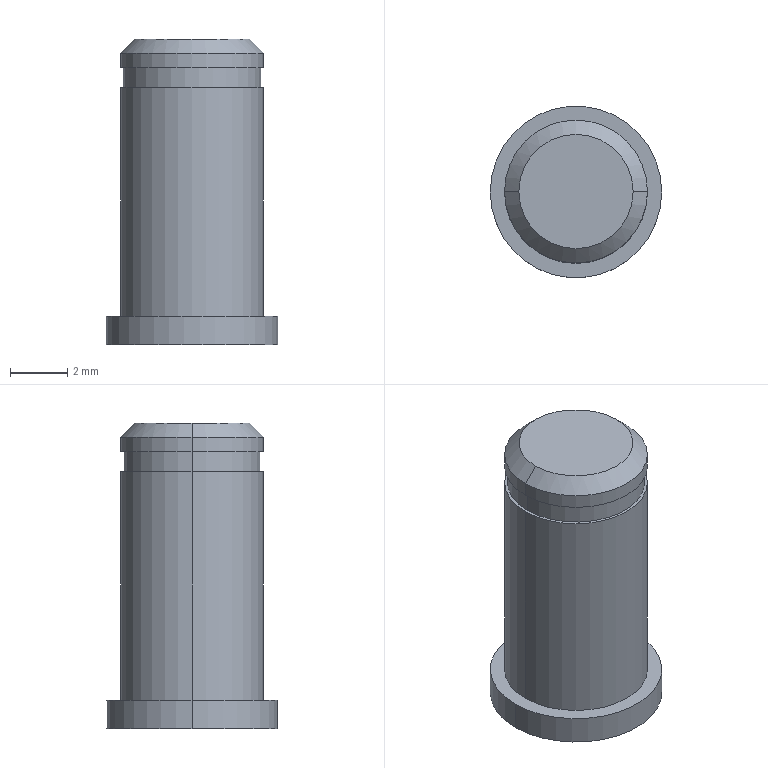Part | STEP file | PN_0105 Mount electronic clip sensor 3 | 1 solid | 15 faces | box 6 x 6 x 10.7 mm | volume 215.823 mm3 | cylinder 8 | plane 5 | cone 2 | commonest cylinder face diameters 5 x4 4.8 x2 6 x2
STEP:
#1=CARTESIAN_POINT('',(0.,0.,0.));
#2=DIRECTION('',(0.,0.,1.));
#3=DIRECTION('',(1.,0.,0.));
#4=AXIS2_PLACEMENT_3D('',#1,#2,#3);
#5=CARTESIAN_POINT('',(2.,0.,10.7));
#6=VERTEX_POINT('',#5);
#7=CARTESIAN_POINT('',(-2.,0.,10.7));
#8=VERTEX_POINT('',#7);
#9=CARTESIAN_POINT('',(0.,0.,10.7));
#10=DIRECTION('',(0.,0.,1.));
#11=DIRECTION('',(1.,0.,0.));
#12=AXIS2_PLACEMENT_3D('',#9,#10,#11);
#13=CIRCLE('',#12,2.);
#14=CARTESIAN_POINT('',(0.,0.,10.7));
#15=DIRECTION('',(0.,0.,-1.));
#16=DIRECTION('',(-1.,0.,0.));
#17=AXIS2_PLACEMENT_3D('',#14,#15,#16);
#18=CONICAL_SURFACE('',#17,2.,0.7854);
#19=CARTESIAN_POINT('',(3.142,0.));
#20=DIRECTION('',(-1.,0.));
#21=VECTOR('',#20,1.);
#22=LINE('',#19,#21);
#23=(GEOMETRIC_REPRESENTATION_CONTEXT(2)PARAMETRIC_REPRESENTATION_CONTEXT()REPRESENTATION_CONTEXT('',''));
#24=DEFINITIONAL_REPRESENTATION('',(#22),#23);
#25=PCURVE('',#18,#24);
#26=CARTESIAN_POINT('',(0.,0.,10.7));
#27=DIRECTION('',(0.,0.,1.));
#28=DIRECTION('',(1.,0.,0.));
#29=AXIS2_PLACEMENT_3D('',#26,#27,#28);
#30=PLANE('',#29);
#31=CARTESIAN_POINT('',(0.,0.));
#32=DIRECTION('',(1.,0.));
#33=AXIS2_PLACEMENT_2D('',#31,#32);
#34=CIRCLE('',#33,2.);
#35=(GEOMETRIC_REPRESENTATION_CONTEXT(2)PARAMETRIC_REPRESENTATION_CONTEXT()REPRESENTATION_CONTEXT('',''));
#36=DEFINITIONAL_REPRESENTATION('',(#34),#35);
#37=PCURVE('',#30,#36);
#38=SURFACE_CURVE('',#13,(#25,#37),.PCURVE_S1.);
#39=EDGE_CURVE('',#6,#8,#38,.T.);
#40=ORIENTED_EDGE('',*,*,#39,.F.);
#41=CARTESIAN_POINT('',(2.5,0.,10.2));
#42=VERTEX_POINT('',#41);
#43=CARTESIAN_POINT('',(2.,0.,10.7));
#44=DIRECTION('',(0.7071,0.,-0.7071));
#45=VECTOR('',#44,1.);
#46=LINE('',#43,#45);
#47=CARTESIAN_POINT('',(3.142,0.));
#48=DIRECTION('',(0.,1.));
#49=VECTOR('',#48,1.);
#50=LINE('',#47,#49);
#51=(GEOMETRIC_REPRESENTATION_CONTEXT(2)PARAMETRIC_REPRESENTATION_CONTEXT()REPRESENTATION_CONTEXT('',''));
#52=DEFINITIONAL_REPRESENTATION('',(#50),#51);
#53=PCURVE('',#18,#52);
#54=CARTESIAN_POINT('',(0.,0.,10.7));
#55=DIRECTION('',(0.,0.,-1.));
#56=DIRECTION('',(-1.,0.,0.));
#57=AXIS2_PLACEMENT_3D('',#54,#55,#56);
#58=CONICAL_SURFACE('',#57,2.,0.7854);
#59=CARTESIAN_POINT('',(3.142,0.));
#60=DIRECTION('',(0.,1.));
#61=VECTOR('',#60,1.);
#62=LINE('',#59,#61);
#63=(GEOMETRIC_REPRESENTATION_CONTEXT(2)PARAMETRIC_REPRESENTATION_CONTEXT()REPRESENTATION_CONTEXT('',''));
#64=DEFINITIONAL_REPRESENTATION('',(#62),#63);
#65=PCURVE('',#58,#64);
#66=SURFACE_CURVE('',#46,(#53,#65),.PCURVE_S1.);
#67=EDGE_CURVE('',#6,#42,#66,.T.);
#68=ORIENTED_EDGE('',*,*,#67,.T.);
#69=CARTESIAN_POINT('',(-2.5,0.,10.2));
#70=VERTEX_POINT('',#69);
#71=CARTESIAN_POINT('',(0.,0.,10.2));
#72=DIRECTION('',(0.,0.,-1.));
#73=DIRECTION('',(1.,0.,0.));
#74=AXIS2_PLACEMENT_3D('',#71,#72,#73);
#75=CIRCLE('',#74,2.5);
#76=CARTESIAN_POINT('',(-3.142,0.5));
#77=DIRECTION('',(1.,0.));
#78=VECTOR('',#77,1.);
#79=LINE('',#76,#78);
#80=(GEOMETRIC_REPRESENTATION_CONTEXT(2)PARAMETRIC_REPRESENTATION_CONTEXT()REPRESENTATION_CONTEXT('',''));
#81=DEFINITIONAL_REPRESENTATION('',(#79),#80);
#82=PCURVE('',#18,#81);
#83=CARTESIAN_POINT('',(0.,0.,10.7));
#84=DIRECTION('',(0.,0.,-1.));
#85=DIRECTION('',(-1.,0.,0.));
#86=AXIS2_PLACEMENT_3D('',#83,#84,#85);
#87=CYLINDRICAL_SURFACE('',#86,2.5);
#88=CARTESIAN_POINT('',(-3.142,0.5));
#89=DIRECTION('',(1.,0.));
#90=VECTOR('',#89,1.);
#91=LINE('',#88,#90);
#92=(GEOMETRIC_REPRESENTATION_CONTEXT(2)PARAMETRIC_REPRESENTATION_CONTEXT()REPRESENTATION_CONTEXT('',''));
#93=DEFINITIONAL_REPRESENTATION('',(#91),#92);
#94=PCURVE('',#87,#93);
#95=SURFACE_CURVE('',#75,(#82,#94),.PCURVE_S1.);
#96=EDGE_CURVE('',#70,#42,#95,.T.);
#97=ORIENTED_EDGE('',*,*,#96,.F.);
#98=CARTESIAN_POINT('',(-2.,0.,10.7));
#99=DIRECTION('',(-0.7071,0.,-0.7071));
#100=VECTOR('',#99,1.);
#101=LINE('',#98,#100);
#102=CARTESIAN_POINT('',(0.,0.));
#103=DIRECTION('',(0.,1.));
#104=VECTOR('',#103,1.);
#105=LINE('',#102,#104);
#106=(GEOMETRIC_REPRESENTATION_CONTEXT(2)PARAMETRIC_REPRESENTATION_CONTEXT()REPRESENTATION_CONTEXT('',''));
#107=DEFINITIONAL_REPRESENTATION('',(#105),#106);
#108=PCURVE('',#18,#107);
#109=CARTESIAN_POINT('',(6.283,0.));
#110=DIRECTION('',(0.,1.));
#111=VECTOR('',#110,1.);
#112=LINE('',#109,#111);
#113=(GEOMETRIC_REPRESENTATION_CONTEXT(2)PARAMETRIC_REPRESENTATION_CONTEXT()REPRESENTATION_CONTEXT('',''));
#114=DEFINITIONAL_REPRESENTATION('',(#112),#113);
#115=PCURVE('',#58,#114);
#116=SURFACE_CURVE('',#101,(#108,#115),.PCURVE_S1.);
#117=EDGE_CURVE('',#8,#70,#116,.T.);
#118=ORIENTED_EDGE('',*,*,#117,.F.);
#119=EDGE_LOOP('',(#40,#68,#97,#118));
#120=FACE_BOUND('',#119,.T.);
#121=ADVANCED_FACE('',(#120),#18,.T.);
#122=ORIENTED_EDGE('',*,*,#96,.T.);
#123=CARTESIAN_POINT('',(2.5,0.,9.7));
#124=VERTEX_POINT('',#123);
#125=CARTESIAN_POINT('',(2.5,0.,10.7));
#126=DIRECTION('',(0.,0.,-1.));
#127=VECTOR('',#126,1.);
#128=LINE('',#125,#127);
#129=CARTESIAN_POINT('',(3.142,0.));
#130=DIRECTION('',(0.,1.));
#131=VECTOR('',#130,1.);
#132=LINE('',#129,#131);
#133=(GEOMETRIC_REPRESENTATION_CONTEXT(2)PARAMETRIC_REPRESENTATION_CONTEXT()REPRESENTATION_CONTEXT('',''));
#134=DEFINITIONAL_REPRESENTATION('',(#132),#133);
#135=PCURVE('',#87,#134);
#136=CARTESIAN_POINT('',(0.,0.,10.7));
#137=DIRECTION('',(0.,0.,-1.));
#138=DIRECTION('',(-1.,0.,0.));
#139=AXIS2_PLACEMENT_3D('',#136,#137,#138);
#140=CYLINDRICAL_SURFACE('',#139,2.5);
#141=CARTESIAN_POINT('',(3.142,0.));
#142=DIRECTION('',(0.,1.));
#143=VECTOR('',#142,1.);
#144=LINE('',#141,#143);
#145=(GEOMETRIC_REPRESENTATION_CONTEXT(2)PARAMETRIC_REPRESENTATION_CONTEXT()REPRESENTATION_CONTEXT('',''));
#146=DEFINITIONAL_REPRESENTATION('',(#144),#145);
#147=PCURVE('',#140,#146);
#148=SURFACE_CURVE('',#128,(#135,#147),.PCURVE_S1.);
#149=EDGE_CURVE('',#42,#124,#148,.T.);
#150=ORIENTED_EDGE('',*,*,#149,.T.);
#151=CARTESIAN_POINT('',(-2.5,0.,9.7));
#152=VERTEX_POINT('',#151);
#153=CARTESIAN_POINT('',(0.,0.,9.7));
#154=DIRECTION('',(0.,0.,1.));
#155=DIRECTION('',(1.,0.,0.));
#156=AXIS2_PLACEMENT_3D('',#153,#154,#155);
#157=CIRCLE('',#156,2.5);
#158=CARTESIAN_POINT('',(3.142,1.));
#159=DIRECTION('',(-1.,0.));
#160=VECTOR('',#159,1.);
#161=LINE('',#158,#160);
#162=(GEOMETRIC_REPRESENTATION_CONTEXT(2)PARAMETRIC_REPRESENTATION_CONTEXT()REPRESENTATION_CONTEXT('',''));
#163=DEFINITIONAL_REPRESENTATION('',(#161),#162);
#164=PCURVE('',#87,#163);
#165=CARTESIAN_POINT('',(0.,0.,9.7));
#166=DIRECTION('',(0.,0.,1.));
#167=DIRECTION('',(1.,0.,0.));
#168=AXIS2_PLACEMENT_3D('',#165,#166,#167);
#169=PLANE('',#168);
#170=CARTESIAN_POINT('',(0.,0.));
#171=DIRECTION('',(1.,0.));
#172=AXIS2_PLACEMENT_2D('',#170,#171);
#173=CIRCLE('',#172,2.5);
#174=(GEOMETRIC_REPRESENTATION_CONTEXT(2)PARAMETRIC_REPRESENTATION_CONTEXT()REPRESENTATION_CONTEXT('',''));
#175=DEFINITIONAL_REPRESENTATION('',(#173),#174);
#176=PCURVE('',#169,#175);
#177=SURFACE_CURVE('',#157,(#164,#176),.PCURVE_S1.);
#178=EDGE_CURVE('',#124,#152,#177,.T.);
#179=ORIENTED_EDGE('',*,*,#178,.T.);
#180=CARTESIAN_POINT('',(-2.5,0.,10.7));
#181=DIRECTION('',(0.,0.,-1.));
#182=VECTOR('',#181,1.);
#183=LINE('',#180,#182);
#184=CARTESIAN_POINT('',(0.,0.));
#185=DIRECTION('',(0.,1.));
#186=VECTOR('',#185,1.);
#187=LINE('',#184,#186);
#188=(GEOMETRIC_REPRESENTATION_CONTEXT(2)PARAMETRIC_REPRESENTATION_CONTEXT()REPRESENTATION_CONTEXT('',''));
#189=DEFINITIONAL_REPRESENTATION('',(#187),#188);
#190=PCURVE('',#87,#189);
#191=CARTESIAN_POINT('',(6.283,0.));
#192=DIRECTION('',(0.,1.));
#193=VECTOR('',#192,1.);
#194=LINE('',#191,#193);
#195=(GEOMETRIC_REPRESENTATION_CONTEXT(2)PARAMETRIC_REPRESENTATION_CONTEXT()REPRESENTATION_CONTEXT('',''));
#196=DEFINITIONAL_REPRESENTATION('',(#194),#195);
#197=PCURVE('',#140,#196);
#198=SURFACE_CURVE('',#183,(#190,#197),.PCURVE_S1.);
#199=EDGE_CURVE('',#70,#152,#198,.T.);
#200=ORIENTED_EDGE('',*,*,#199,.F.);
#201=EDGE_LOOP('',(#122,#150,#179,#200));
#202=FACE_BOUND('',#201,.T.);
#203=ADVANCED_FACE('',(#202),#87,.T.);
#204=CARTESIAN_POINT('',(2.4,0.,9.7));
#205=VERTEX_POINT('',#204);
#206=CARTESIAN_POINT('',(-2.4,0.,9.7));
#207=VERTEX_POINT('',#206);
#208=CARTESIAN_POINT('',(0.,0.,9.7));
#209=DIRECTION('',(0.,0.,1.));
#210=DIRECTION('',(1.,0.,0.));
#211=AXIS2_PLACEMENT_3D('',#208,#209,#210);
#212=CIRCLE('',#211,2.4);
#213=CARTESIAN_POINT('',(0.,0.,9.7));
#214=DIRECTION('',(0.,0.,-1.));
#215=DIRECTION('',(-1.,0.,0.));
#216=AXIS2_PLACEMENT_3D('',#213,#214,#215);
#217=CYLINDRICAL_SURFACE('',#216,2.4);
#218=CARTESIAN_POINT('',(3.142,0.));
#219=DIRECTION('',(-1.,0.));
#220=VECTOR('',#219,1.);
#221=LINE('',#218,#220);
#222=(GEOMETRIC_REPRESENTATION_CONTEXT(2)PARAMETRIC_REPRESENTATION_CONTEXT()REPRESENTATION_CONTEXT('',''));
#223=DEFINITIONAL_REPRESENTATION('',(#221),#222);
#224=PCURVE('',#217,#223);
#225=CARTESIAN_POINT('',(0.,0.));
#226=DIRECTION('',(1.,0.));
#227=AXIS2_PLACEMENT_2D('',#225,#226);
#228=CIRCLE('',#227,2.4);
#229=(GEOMETRIC_REPRESENTATION_CONTEXT(2)PARAMETRIC_REPRESENTATION_CONTEXT()REPRESENTATION_CONTEXT('',''));
#230=DEFINITIONAL_REPRESENTATION('',(#228),#229);
#231=PCURVE('',#169,#230);
#232=SURFACE_CURVE('',#212,(#224,#231),.PCURVE_S1.);
#233=EDGE_CURVE('',#205,#207,#232,.T.);
#234=ORIENTED_EDGE('',*,*,#233,.F.);
#235=CARTESIAN_POINT('',(2.4,0.,9.));
#236=VERTEX_POINT('',#235);
#237=CARTESIAN_POINT('',(2.4,0.,9.7));
#238=DIRECTION('',(0.,0.,-1.));
#239=VECTOR('',#238,1.);
#240=LINE('',#237,#239);
#241=CARTESIAN_POINT('',(3.142,0.));
#242=DIRECTION('',(0.,1.));
#243=VECTOR('',#242,1.);
#244=LINE('',#241,#243);
#245=(GEOMETRIC_REPRESENTATION_CONTEXT(2)PARAMETRIC_REPRESENTATION_CONTEXT()REPRESENTATION_CONTEXT('',''));
#246=DEFINITIONAL_REPRESENTATION('',(#244),#245);
#247=PCURVE('',#217,#246);
#248=CARTESIAN_POINT('',(0.,0.,9.7));
#249=DIRECTION('',(0.,0.,-1.));
#250=DIRECTION('',(-1.,0.,0.));
#251=AXIS2_PLACEMENT_3D('',#248,#249,#250);
#252=CYLINDRICAL_SURFACE('',#251,2.4);
#253=CARTESIAN_POINT('',(3.142,0.));
#254=DIRECTION('',(0.,1.));
#255=VECTOR('',#254,1.);
#256=LINE('',#253,#255);
#257=(GEOMETRIC_REPRESENTATION_CONTEXT(2)PARAMETRIC_REPRESENTATION_CONTEXT()REPRESENTATION_CONTEXT('',''));
#258=DEFINITIONAL_REPRESENTATION('',(#256),#257);
#259=PCURVE('',#252,#258);
#260=SURFACE_CURVE('',#240,(#247,#259),.PCURVE_S1.);
#261=EDGE_CURVE('',#205,#236,#260,.T.);
#262=ORIENTED_EDGE('',*,*,#261,.T.);
#263=CARTESIAN_POINT('',(-2.4,0.,9.));
#264=VERTEX_POINT('',#263);
#265=CARTESIAN_POINT('',(0.,0.,9.));
#266=DIRECTION('',(0.,0.,1.));
#267=DIRECTION('',(1.,0.,0.));
#268=AXIS2_PLACEMENT_3D('',#265,#266,#267);
#269=CIRCLE('',#268,2.4);
#270=CARTESIAN_POINT('',(3.142,0.7));
#271=DIRECTION('',(-1.,0.));
#272=VECTOR('',#271,1.);
#273=LINE('',#270,#272);
#274=(GEOMETRIC_REPRESENTATION_CONTEXT(2)PARAMETRIC_REPRESENTATION_CONTEXT()REPRESENTATION_CONTEXT('',''));
#275=DEFINITIONAL_REPRESENTATION('',(#273),#274);
#276=PCURVE('',#217,#275);
#277=CARTESIAN_POINT('',(0.,0.,9.));
#278=DIRECTION('',(0.,0.,1.));
#279=DIRECTION('',(1.,0.,0.));
#280=AXIS2_PLACEMENT_3D('',#277,#278,#279);
#281=PLANE('',#280);
#282=CARTESIAN_POINT('',(0.,0.));
#283=DIRECTION('',(1.,0.));
#284=AXIS2_PLACEMENT_2D('',#282,#283);
#285=CIRCLE('',#284,2.4);
#286=(GEOMETRIC_REPRESENTATION_CONTEXT(2)PARAMETRIC_REPRESENTATION_CONTEXT()REPRESENTATION_CONTEXT('',''));
#287=DEFINITIONAL_REPRESENTATION('',(#285),#286);
#288=PCURVE('',#281,#287);
#289=SURFACE_CURVE('',#269,(#276,#288),.PCURVE_S1.);
#290=EDGE_CURVE('',#236,#264,#289,.T.);
#291=ORIENTED_EDGE('',*,*,#290,.T.);
#292=CARTESIAN_POINT('',(-2.4,0.,9.7));
#293=DIRECTION('',(0.,0.,-1.));
#294=VECTOR('',#293,1.);
#295=LINE('',#292,#294);
#296=CARTESIAN_POINT('',(0.,0.));
#297=DIRECTION('',(0.,1.));
#298=VECTOR('',#297,1.);
#299=LINE('',#296,#298);
#300=(GEOMETRIC_REPRESENTATION_CONTEXT(2)PARAMETRIC_REPRESENTATION_CONTEXT()REPRESENTATION_CONTEXT('',''));
#301=DEFINITIONAL_REPRESENTATION('',(#299),#300);
#302=PCURVE('',#217,#301);
#303=CARTESIAN_POINT('',(6.283,0.));
#304=DIRECTION('',(0.,1.));
#305=VECTOR('',#304,1.);
#306=LINE('',#303,#305);
#307=(GEOMETRIC_REPRESENTATION_CONTEXT(2)PARAMETRIC_REPRESENTATION_CONTEXT()REPRESENTATION_CONTEXT('',''));
#308=DEFINITIONAL_REPRESENTATION('',(#306),#307);
#309=PCURVE('',#252,#308);
#310=SURFACE_CURVE('',#295,(#302,#309),.PCURVE_S1.);
#311=EDGE_CURVE('',#207,#264,#310,.T.);
#312=ORIENTED_EDGE('',*,*,#311,.F.);
#313=EDGE_LOOP('',(#234,#262,#291,#312));
#314=FACE_BOUND('',#313,.T.);
#315=ADVANCED_FACE('',(#314),#217,.T.);
#316=CARTESIAN_POINT('',(2.5,0.,9.));
#317=VERTEX_POINT('',#316);
#318=CARTESIAN_POINT('',(-2.5,0.,9.));
#319=VERTEX_POINT('',#318);
#320=CARTESIAN_POINT('',(0.,0.,9.));
#321=DIRECTION('',(0.,0.,1.));
#322=DIRECTION('',(1.,0.,0.));
#323=AXIS2_PLACEMENT_3D('',#320,#321,#322);
#324=CIRCLE('',#323,2.5);
#325=CARTESIAN_POINT('',(0.,0.,9.));
#326=DIRECTION('',(0.,0.,-1.));
#327=DIRECTION('',(-1.,0.,0.));
#328=AXIS2_PLACEMENT_3D('',#325,#326,#327);
#329=CYLINDRICAL_SURFACE('',#328,2.5);
#330=CARTESIAN_POINT('',(3.142,0.));
#331=DIRECTION('',(-1.,0.));
#332=VECTOR('',#331,1.);
#333=LINE('',#330,#332);
#334=(GEOMETRIC_REPRESENTATION_CONTEXT(2)PARAMETRIC_REPRESENTATION_CONTEXT()REPRESENTATION_CONTEXT('',''));
#335=DEFINITIONAL_REPRESENTATION('',(#333),#334);
#336=PCURVE('',#329,#335);
#337=CARTESIAN_POINT('',(0.,0.));
#338=DIRECTION('',(1.,0.));
#339=AXIS2_PLACEMENT_2D('',#337,#338);
#340=CIRCLE('',#339,2.5);
#341=(GEOMETRIC_REPRESENTATION_CONTEXT(2)PARAMETRIC_REPRESENTATION_CONTEXT()REPRESENTATION_CONTEXT('',''));
#342=DEFINITIONAL_REPRESENTATION('',(#340),#341);
#343=PCURVE('',#281,#342);
#344=SURFACE_CURVE('',#324,(#336,#343),.PCURVE_S1.);
#345=EDGE_CURVE('',#317,#319,#344,.T.);
#346=ORIENTED_EDGE('',*,*,#345,.F.);
#347=CARTESIAN_POINT('',(2.5,0.,1.));
#348=VERTEX_POINT('',#347);
#349=CARTESIAN_POINT('',(2.5,0.,9.));
#350=DIRECTION('',(0.,0.,-1.));
#351=VECTOR('',#350,1.);
#352=LINE('',#349,#351);
#353=CARTESIAN_POINT('',(3.142,0.));
#354=DIRECTION('',(0.,1.));
#355=VECTOR('',#354,1.);
#356=LINE('',#353,#355);
#357=(GEOMETRIC_REPRESENTATION_CONTEXT(2)PARAMETRIC_REPRESENTATION_CONTEXT()REPRESENTATION_CONTEXT('',''));
#358=DEFINITIONAL_REPRESENTATION('',(#356),#357);
#359=PCURVE('',#329,#358);
#360=CARTESIAN_POINT('',(0.,0.,9.));
#361=DIRECTION('',(0.,0.,-1.));
#362=DIRECTION('',(-1.,0.,0.));
#363=AXIS2_PLACEMENT_3D('',#360,#361,#362);
#364=CYLINDRICAL_SURFACE('',#363,2.5);
#365=CARTESIAN_POINT('',(3.142,0.));
#366=DIRECTION('',(0.,1.));
#367=VECTOR('',#366,1.);
#368=LINE('',#365,#367);
#369=(GEOMETRIC_REPRESENTATION_CONTEXT(2)PARAMETRIC_REPRESENTATION_CONTEXT()REPRESENTATION_CONTEXT('',''));
#370=DEFINITIONAL_REPRESENTATION('',(#368),#369);
#371=PCURVE('',#364,#370);
#372=SURFACE_CURVE('',#352,(#359,#371),.PCURVE_S1.);
#373=EDGE_CURVE('',#317,#348,#372,.T.);
#374=ORIENTED_EDGE('',*,*,#373,.T.);
#375=CARTESIAN_POINT('',(-2.5,0.,1.));
#376=VERTEX_POINT('',#375);
#377=CARTESIAN_POINT('',(0.,0.,1.));
#378=DIRECTION('',(0.,0.,1.));
#379=DIRECTION('',(1.,0.,0.));
#380=AXIS2_PLACEMENT_3D('',#377,#378,#379);
#381=CIRCLE('',#380,2.5);
#382=CARTESIAN_POINT('',(3.142,8.));
#383=DIRECTION('',(-1.,0.));
#384=VECTOR('',#383,1.);
#385=LINE('',#382,#384);
#386=(GEOMETRIC_REPRESENTATION_CONTEXT(2)PARAMETRIC_REPRESENTATION_CONTEXT()REPRESENTATION_CONTEXT('',''));
#387=DEFINITIONAL_REPRESENTATION('',(#385),#386);
#388=PCURVE('',#329,#387);
#389=CARTESIAN_POINT('',(0.,0.,1.));
#390=DIRECTION('',(0.,0.,1.));
#391=DIRECTION('',(1.,0.,0.));
#392=AXIS2_PLACEMENT_3D('',#389,#390,#391);
#393=PLANE('',#392);
#394=CARTESIAN_POINT('',(0.,0.));
#395=DIRECTION('',(1.,0.));
#396=AXIS2_PLACEMENT_2D('',#394,#395);
#397=CIRCLE('',#396,2.5);
#398=(GEOMETRIC_REPRESENTATION_CONTEXT(2)PARAMETRIC_REPRESENTATION_CONTEXT()REPRESENTATION_CONTEXT('',''));
#399=DEFINITIONAL_REPRESENTATION('',(#397),#398);
#400=PCURVE('',#393,#399);
#401=SURFACE_CURVE('',#381,(#388,#400),.PCURVE_S1.);
#402=EDGE_CURVE('',#348,#376,#401,.T.);
#403=ORIENTED_EDGE('',*,*,#402,.T.);
#404=CARTESIAN_POINT('',(-2.5,0.,9.));
#405=DIRECTION('',(0.,0.,-1.));
#406=VECTOR('',#405,1.);
#407=LINE('',#404,#406);
#408=CARTESIAN_POINT('',(0.,0.));
#409=DIRECTION('',(0.,1.));
#410=VECTOR('',#409,1.);
#411=LINE('',#408,#410);
#412=(GEOMETRIC_REPRESENTATION_CONTEXT(2)PARAMETRIC_REPRESENTATION_CONTEXT()REPRESENTATION_CONTEXT('',''));
#413=DEFINITIONAL_REPRESENTATION('',(#411),#412);
#414=PCURVE('',#329,#413);
#415=CARTESIAN_POINT('',(6.283,0.));
#416=DIRECTION('',(0.,1.));
#417=VECTOR('',#416,1.);
#418=LINE('',#415,#417);
#419=(GEOMETRIC_REPRESENTATION_CONTEXT(2)PARAMETRIC_REPRESENTATION_CONTEXT()REPRESENTATION_CONTEXT('',''));
#420=DEFINITIONAL_REPRESENTATION('',(#418),#419);
#421=PCURVE('',#364,#420);
#422=SURFACE_CURVE('',#407,(#414,#421),.PCURVE_S1.);
#423=EDGE_CURVE('',#319,#376,#422,.T.);
#424=ORIENTED_EDGE('',*,*,#423,.F.);
#425=EDGE_LOOP('',(#346,#374,#403,#424));
#426=FACE_BOUND('',#425,.T.);
#427=ADVANCED_FACE('',(#426),#329,.T.);
#428=CARTESIAN_POINT('',(3.,0.,1.));
#429=VERTEX_POINT('',#428);
#430=CARTESIAN_POINT('',(-3.,0.,1.));
#431=VERTEX_POINT('',#430);
#432=CARTESIAN_POINT('',(0.,0.,1.));
#433=DIRECTION('',(0.,0.,1.));
#434=DIRECTION('',(1.,0.,0.));
#435=AXIS2_PLACEMENT_3D('',#432,#433,#434);
#436=CIRCLE('',#435,3.);
#437=CARTESIAN_POINT('',(0.,0.,1.));
#438=DIRECTION('',(0.,0.,-1.));
#439=DIRECTION('',(-1.,0.,0.));
#440=AXIS2_PLACEMENT_3D('',#437,#438,#439);
#441=CYLINDRICAL_SURFACE('',#440,3.);
#442=CARTESIAN_POINT('',(3.142,0.));
#443=DIRECTION('',(-1.,0.));
#444=VECTOR('',#443,1.);
#445=LINE('',#442,#444);
#446=(GEOMETRIC_REPRESENTATION_CONTEXT(2)PARAMETRIC_REPRESENTATION_CONTEXT()REPRESENTATION_CONTEXT('',''));
#447=DEFINITIONAL_REPRESENTATION('',(#445),#446);
#448=PCURVE('',#441,#447);
#449=CARTESIAN_POINT('',(0.,0.));
#450=DIRECTION('',(1.,0.));
#451=AXIS2_PLACEMENT_2D('',#449,#450);
#452=CIRCLE('',#451,3.);
#453=(GEOMETRIC_REPRESENTATION_CONTEXT(2)PARAMETRIC_REPRESENTATION_CONTEXT()REPRESENTATION_CONTEXT('',''));
#454=DEFINITIONAL_REPRESENTATION('',(#452),#453);
#455=PCURVE('',#393,#454);
#456=SURFACE_CURVE('',#436,(#448,#455),.PCURVE_S1.);
#457=EDGE_CURVE('',#429,#431,#456,.T.);
#458=ORIENTED_EDGE('',*,*,#457,.F.);
#459=CARTESIAN_POINT('',(3.,0.,0.));
#460=VERTEX_POINT('',#459);
#461=CARTESIAN_POINT('',(3.,0.,1.));
#462=DIRECTION('',(0.,0.,-1.));
#463=VECTOR('',#462,1.);
#464=LINE('',#461,#463);
#465=CARTESIAN_POINT('',(3.142,0.));
#466=DIRECTION('',(0.,1.));
#467=VECTOR('',#466,1.);
#468=LINE('',#465,#467);
#469=(GEOMETRIC_REPRESENTATION_CONTEXT(2)PARAMETRIC_REPRESENTATION_CONTEXT()REPRESENTATION_CONTEXT('',''));
#470=DEFINITIONAL_REPRESENTATION('',(#468),#469);
#471=PCURVE('',#441,#470);
#472=CARTESIAN_POINT('',(0.,0.,1.));
#473=DIRECTION('',(0.,0.,-1.));
#474=DIRECTION('',(-1.,0.,0.));
#475=AXIS2_PLACEMENT_3D('',#472,#473,#474);
#476=CYLINDRICAL_SURFACE('',#475,3.);
#477=CARTESIAN_POINT('',(3.142,0.));
#478=DIRECTION('',(0.,1.));
#479=VECTOR('',#478,1.);
#480=LINE('',#477,#479);
#481=(GEOMETRIC_REPRESENTATION_CONTEXT(2)PARAMETRIC_REPRESENTATION_CONTEXT()REPRESENTATION_CONTEXT('',''));
#482=DEFINITIONAL_REPRESENTATION('',(#480),#481);
#483=PCURVE('',#476,#482);
#484=SURFACE_CURVE('',#464,(#471,#483),.PCURVE_S1.);
#485=EDGE_CURVE('',#429,#460,#484,.T.);
#486=ORIENTED_EDGE('',*,*,#485,.T.);
#487=CARTESIAN_POINT('',(-3.,0.,0.));
#488=VERTEX_POINT('',#487);
#489=CARTESIAN_POINT('',(0.,0.,0.));
#490=DIRECTION('',(0.,0.,1.));
#491=DIRECTION('',(1.,0.,0.));
#492=AXIS2_PLACEMENT_3D('',#489,#490,#491);
#493=CIRCLE('',#492,3.);
#494=CARTESIAN_POINT('',(3.142,1.));
#495=DIRECTION('',(-1.,0.));
#496=VECTOR('',#495,1.);
#497=LINE('',#494,#496);
#498=(GEOMETRIC_REPRESENTATION_CONTEXT(2)PARAMETRIC_REPRESENTATION_CONTEXT()REPRESENTATION_CONTEXT('',''));
#499=DEFINITIONAL_REPRESENTATION('',(#497),#498);
#500=PCURVE('',#441,#499);
#501=CARTESIAN_POINT('',(0.,0.,0.));
#502=DIRECTION('',(0.,0.,1.));
#503=DIRECTION('',(1.,0.,0.));
#504=AXIS2_PLACEMENT_3D('',#501,#502,#503);
#505=PLANE('',#504);
#506=CARTESIAN_POINT('',(0.,0.));
#507=DIRECTION('',(1.,0.));
#508=AXIS2_PLACEMENT_2D('',#506,#507);
#509=CIRCLE('',#508,3.);
#510=(GEOMETRIC_REPRESENTATION_CONTEXT(2)PARAMETRIC_REPRESENTATION_CONTEXT()REPRESENTATION_CONTEXT('',''));
#511=DEFINITIONAL_REPRESENTATION('',(#509),#510);
#512=PCURVE('',#505,#511);
#513=SURFACE_CURVE('',#493,(#500,#512),.PCURVE_S1.);
#514=EDGE_CURVE('',#460,#488,#513,.T.);
#515=ORIENTED_EDGE('',*,*,#514,.T.);
#516=CARTESIAN_POINT('',(-3.,0.,1.));
#517=DIRECTION('',(0.,0.,-1.));
#518=VECTOR('',#517,1.);
#519=LINE('',#516,#518);
#520=CARTESIAN_POINT('',(0.,0.));
#521=DIRECTION('',(0.,1.));
#522=VECTOR('',#521,1.);
#523=LINE('',#520,#522);
#524=(GEOMETRIC_REPRESENTATION_CONTEXT(2)PARAMETRIC_REPRESENTATION_CONTEXT()REPRESENTATION_CONTEXT('',''));
#525=DEFINITIONAL_REPRESENTATION('',(#523),#524);
#526=PCURVE('',#441,#525);
#527=CARTESIAN_POINT('',(6.283,0.));
#528=DIRECTION('',(0.,1.));
#529=VECTOR('',#528,1.);
#530=LINE('',#527,#529);
#531=(GEOMETRIC_REPRESENTATION_CONTEXT(2)PARAMETRIC_REPRESENTATION_CONTEXT()REPRESENTATION_CONTEXT('',''));
#532=DEFINITIONAL_REPRESENTATION('',(#530),#531);
#533=PCURVE('',#476,#532);
#534=SURFACE_CURVE('',#519,(#526,#533),.PCURVE_S1.);
#535=EDGE_CURVE('',#431,#488,#534,.T.);
#536=ORIENTED_EDGE('',*,*,#535,.F.);
#537=EDGE_LOOP('',(#458,#486,#515,#536));
#538=FACE_BOUND('',#537,.T.);
#539=ADVANCED_FACE('',(#538),#441,.T.);
#540=CARTESIAN_POINT('',(0.,0.,9.));
#541=DIRECTION('',(0.,0.,1.));
#542=DIRECTION('',(1.,0.,0.));
#543=AXIS2_PLACEMENT_3D('',#540,#541,#542);
#544=CIRCLE('',#543,2.5);
#545=CARTESIAN_POINT('',(0.,0.));
#546=DIRECTION('',(1.,0.));
#547=AXIS2_PLACEMENT_2D('',#545,#546);
#548=CIRCLE('',#547,2.5);
#549=(GEOMETRIC_REPRESENTATION_CONTEXT(2)PARAMETRIC_REPRESENTATION_CONTEXT()REPRESENTATION_CONTEXT('',''));
#550=DEFINITIONAL_REPRESENTATION('',(#548),#549);
#551=PCURVE('',#281,#550);
#552=CARTESIAN_POINT('',(9.425,0.));
#553=DIRECTION('',(-1.,0.));
#554=VECTOR('',#553,1.);
#555=LINE('',#552,#554);
#556=(GEOMETRIC_REPRESENTATION_CONTEXT(2)PARAMETRIC_REPRESENTATION_CONTEXT()REPRESENTATION_CONTEXT('',''));
#557=DEFINITIONAL_REPRESENTATION('',(#555),#556);
#558=PCURVE('',#364,#557);
#559=SURFACE_CURVE('',#544,(#551,#558),.PCURVE_S1.);
#560=EDGE_CURVE('',#319,#317,#559,.T.);
#561=ORIENTED_EDGE('',*,*,#560,.T.);
#562=ORIENTED_EDGE('',*,*,#345,.T.);
#563=EDGE_LOOP('',(#561,#562));
#564=FACE_BOUND('',#563,.T.);
#565=CARTESIAN_POINT('',(0.,0.,9.));
#566=DIRECTION('',(0.,0.,1.));
#567=DIRECTION('',(1.,0.,0.));
#568=AXIS2_PLACEMENT_3D('',#565,#566,#567);
#569=CIRCLE('',#568,2.4);
#570=CARTESIAN_POINT('',(0.,0.));
#571=DIRECTION('',(1.,0.));
#572=AXIS2_PLACEMENT_2D('',#570,#571);
#573=CIRCLE('',#572,2.4);
#574=(GEOMETRIC_REPRESENTATION_CONTEXT(2)PARAMETRIC_REPRESENTATION_CONTEXT()REPRESENTATION_CONTEXT('',''));
#575=DEFINITIONAL_REPRESENTATION('',(#573),#574);
#576=PCURVE('',#281,#575);
#577=CARTESIAN_POINT('',(9.425,0.7));
#578=DIRECTION('',(-1.,0.));
#579=VECTOR('',#578,1.);
#580=LINE('',#577,#579);
#581=(GEOMETRIC_REPRESENTATION_CONTEXT(2)PARAMETRIC_REPRESENTATION_CONTEXT()REPRESENTATION_CONTEXT('',''));
#582=DEFINITIONAL_REPRESENTATION('',(#580),#581);
#583=PCURVE('',#252,#582);
#584=SURFACE_CURVE('',#569,(#576,#583),.PCURVE_S1.);
#585=EDGE_CURVE('',#264,#236,#584,.T.);
#586=ORIENTED_EDGE('',*,*,#585,.F.);
#587=ORIENTED_EDGE('',*,*,#290,.F.);
#588=EDGE_LOOP('',(#586,#587));
#589=FACE_BOUND('',#588,.T.);
#590=ADVANCED_FACE('',(#564,#589),#281,.T.);
#591=CARTESIAN_POINT('',(0.,0.,1.));
#592=DIRECTION('',(0.,0.,1.));
#593=DIRECTION('',(1.,0.,0.));
#594=AXIS2_PLACEMENT_3D('',#591,#592,#593);
#595=CIRCLE('',#594,3.);
#596=CARTESIAN_POINT('',(0.,0.));
#597=DIRECTION('',(1.,0.));
#598=AXIS2_PLACEMENT_2D('',#596,#597);
#599=CIRCLE('',#598,3.);
#600=(GEOMETRIC_REPRESENTATION_CONTEXT(2)PARAMETRIC_REPRESENTATION_CONTEXT()REPRESENTATION_CONTEXT('',''));
#601=DEFINITIONAL_REPRESENTATION('',(#599),#600);
#602=PCURVE('',#393,#601);
#603=CARTESIAN_POINT('',(9.425,0.));
#604=DIRECTION('',(-1.,0.));
#605=VECTOR('',#604,1.);
#606=LINE('',#603,#605);
#607=(GEOMETRIC_REPRESENTATION_CONTEXT(2)PARAMETRIC_REPRESENTATION_CONTEXT()REPRESENTATION_CONTEXT('',''));
#608=DEFINITIONAL_REPRESENTATION('',(#606),#607);
#609=PCURVE('',#476,#608);
#610=SURFACE_CURVE('',#595,(#602,#609),.PCURVE_S1.);
#611=EDGE_CURVE('',#431,#429,#610,.T.);
#612=ORIENTED_EDGE('',*,*,#611,.T.);
#613=ORIENTED_EDGE('',*,*,#457,.T.);
#614=EDGE_LOOP('',(#612,#613));
#615=FACE_BOUND('',#614,.T.);
#616=CARTESIAN_POINT('',(0.,0.,1.));
#617=DIRECTION('',(0.,0.,1.));
#618=DIRECTION('',(1.,0.,0.));
#619=AXIS2_PLACEMENT_3D('',#616,#617,#618);
#620=CIRCLE('',#619,2.5);
#621=CARTESIAN_POINT('',(0.,0.));
#622=DIRECTION('',(1.,0.));
#623=AXIS2_PLACEMENT_2D('',#621,#622);
#624=CIRCLE('',#623,2.5);
#625=(GEOMETRIC_REPRESENTATION_CONTEXT(2)PARAMETRIC_REPRESENTATION_CONTEXT()REPRESENTATION_CONTEXT('',''));
#626=DEFINITIONAL_REPRESENTATION('',(#624),#625);
#627=PCURVE('',#393,#626);
#628=CARTESIAN_POINT('',(9.425,8.));
#629=DIRECTION('',(-1.,0.));
#630=VECTOR('',#629,1.);
#631=LINE('',#628,#630);
#632=(GEOMETRIC_REPRESENTATION_CONTEXT(2)PARAMETRIC_REPRESENTATION_CONTEXT()REPRESENTATION_CONTEXT('',''));
#633=DEFINITIONAL_REPRESENTATION('',(#631),#632);
#634=PCURVE('',#364,#633);
#635=SURFACE_CURVE('',#620,(#627,#634),.PCURVE_S1.);
#636=EDGE_CURVE('',#376,#348,#635,.T.);
#637=ORIENTED_EDGE('',*,*,#636,.F.);
#638=ORIENTED_EDGE('',*,*,#402,.F.);
#639=EDGE_LOOP('',(#637,#638));
#640=FACE_BOUND('',#639,.T.);
#641=ADVANCED_FACE('',(#615,#640),#393,.T.);
#642=ORIENTED_EDGE('',*,*,#485,.F.);
#643=ORIENTED_EDGE('',*,*,#611,.F.);
#644=ORIENTED_EDGE('',*,*,#535,.T.);
#645=CARTESIAN_POINT('',(0.,0.,0.));
#646=DIRECTION('',(0.,0.,1.));
#647=DIRECTION('',(1.,0.,0.));
#648=AXIS2_PLACEMENT_3D('',#645,#646,#647);
#649=CIRCLE('',#648,3.);
#650=CARTESIAN_POINT('',(9.425,1.));
#651=DIRECTION('',(-1.,0.));
#652=VECTOR('',#651,1.);
#653=LINE('',#650,#652);
#654=(GEOMETRIC_REPRESENTATION_CONTEXT(2)PARAMETRIC_REPRESENTATION_CONTEXT()REPRESENTATION_CONTEXT('',''));
#655=DEFINITIONAL_REPRESENTATION('',(#653),#654);
#656=PCURVE('',#476,#655);
#657=CARTESIAN_POINT('',(0.,0.));
#658=DIRECTION('',(1.,0.));
#659=AXIS2_PLACEMENT_2D('',#657,#658);
#660=CIRCLE('',#659,3.);
#661=(GEOMETRIC_REPRESENTATION_CONTEXT(2)PARAMETRIC_REPRESENTATION_CONTEXT()REPRESENTATION_CONTEXT('',''));
#662=DEFINITIONAL_REPRESENTATION('',(#660),#661);
#663=PCURVE('',#505,#662);
#664=SURFACE_CURVE('',#649,(#656,#663),.PCURVE_S1.);
#665=EDGE_CURVE('',#488,#460,#664,.T.);
#666=ORIENTED_EDGE('',*,*,#665,.T.);
#667=EDGE_LOOP('',(#642,#643,#644,#666));
#668=FACE_BOUND('',#667,.T.);
#669=ADVANCED_FACE('',(#668),#476,.T.);
#670=ORIENTED_EDGE('',*,*,#665,.F.);
#671=ORIENTED_EDGE('',*,*,#514,.F.);
#672=EDGE_LOOP('',(#670,#671));
#673=FACE_BOUND('',#672,.T.);
#674=ADVANCED_FACE('',(#673),#505,.F.);
#675=ORIENTED_EDGE('',*,*,#373,.F.);
#676=ORIENTED_EDGE('',*,*,#560,.F.);
#677=ORIENTED_EDGE('',*,*,#423,.T.);
#678=ORIENTED_EDGE('',*,*,#636,.T.);
#679=EDGE_LOOP('',(#675,#676,#677,#678));
#680=FACE_BOUND('',#679,.T.);
#681=ADVANCED_FACE('',(#680),#364,.T.);
#682=ORIENTED_EDGE('',*,*,#261,.F.);
#683=CARTESIAN_POINT('',(0.,0.,9.7));
#684=DIRECTION('',(0.,0.,1.));
#685=DIRECTION('',(1.,0.,0.));
#686=AXIS2_PLACEMENT_3D('',#683,#684,#685);
#687=CIRCLE('',#686,2.4);
#688=CARTESIAN_POINT('',(9.425,0.));
#689=DIRECTION('',(-1.,0.));
#690=VECTOR('',#689,1.);
#691=LINE('',#688,#690);
#692=(GEOMETRIC_REPRESENTATION_CONTEXT(2)PARAMETRIC_REPRESENTATION_CONTEXT()REPRESENTATION_CONTEXT('',''));
#693=DEFINITIONAL_REPRESENTATION('',(#691),#692);
#694=PCURVE('',#252,#693);
#695=CARTESIAN_POINT('',(0.,0.));
#696=DIRECTION('',(1.,0.));
#697=AXIS2_PLACEMENT_2D('',#695,#696);
#698=CIRCLE('',#697,2.4);
#699=(GEOMETRIC_REPRESENTATION_CONTEXT(2)PARAMETRIC_REPRESENTATION_CONTEXT()REPRESENTATION_CONTEXT('',''));
#700=DEFINITIONAL_REPRESENTATION('',(#698),#699);
#701=PCURVE('',#169,#700);
#702=SURFACE_CURVE('',#687,(#694,#701),.PCURVE_S1.);
#703=EDGE_CURVE('',#207,#205,#702,.T.);
#704=ORIENTED_EDGE('',*,*,#703,.F.);
#705=ORIENTED_EDGE('',*,*,#311,.T.);
#706=ORIENTED_EDGE('',*,*,#585,.T.);
#707=EDGE_LOOP('',(#682,#704,#705,#706));
#708=FACE_BOUND('',#707,.T.);
#709=ADVANCED_FACE('',(#708),#252,.T.);
#710=CARTESIAN_POINT('',(0.,0.,9.7));
#711=DIRECTION('',(0.,0.,1.));
#712=DIRECTION('',(1.,0.,0.));
#713=AXIS2_PLACEMENT_3D('',#710,#711,#712);
#714=CIRCLE('',#713,2.5);
#715=CARTESIAN_POINT('',(0.,0.));
#716=DIRECTION('',(1.,0.));
#717=AXIS2_PLACEMENT_2D('',#715,#716);
#718=CIRCLE('',#717,2.5);
#719=(GEOMETRIC_REPRESENTATION_CONTEXT(2)PARAMETRIC_REPRESENTATION_CONTEXT()REPRESENTATION_CONTEXT('',''));
#720=DEFINITIONAL_REPRESENTATION('',(#718),#719);
#721=PCURVE('',#169,#720);
#722=CARTESIAN_POINT('',(9.425,1.));
#723=DIRECTION('',(-1.,0.));
#724=VECTOR('',#723,1.);
#725=LINE('',#722,#724);
#726=(GEOMETRIC_REPRESENTATION_CONTEXT(2)PARAMETRIC_REPRESENTATION_CONTEXT()REPRESENTATION_CONTEXT('',''));
#727=DEFINITIONAL_REPRESENTATION('',(#725),#726);
#728=PCURVE('',#140,#727);
#729=SURFACE_CURVE('',#714,(#721,#728),.PCURVE_S1.);
#730=EDGE_CURVE('',#152,#124,#729,.T.);
#731=ORIENTED_EDGE('',*,*,#730,.F.);
#732=ORIENTED_EDGE('',*,*,#178,.F.);
#733=EDGE_LOOP('',(#731,#732));
#734=FACE_BOUND('',#733,.T.);
#735=ORIENTED_EDGE('',*,*,#703,.T.);
#736=ORIENTED_EDGE('',*,*,#233,.T.);
#737=EDGE_LOOP('',(#735,#736));
#738=FACE_BOUND('',#737,.T.);
#739=ADVANCED_FACE('',(#734,#738),#169,.F.);
#740=ORIENTED_EDGE('',*,*,#149,.F.);
#741=CARTESIAN_POINT('',(0.,0.,10.2));
#742=DIRECTION('',(0.,0.,-1.));
#743=DIRECTION('',(1.,0.,0.));
#744=AXIS2_PLACEMENT_3D('',#741,#742,#743);
#745=CIRCLE('',#744,2.5);
#746=CARTESIAN_POINT('',(3.142,0.5));
#747=DIRECTION('',(1.,0.));
#748=VECTOR('',#747,1.);
#749=LINE('',#746,#748);
#750=(GEOMETRIC_REPRESENTATION_CONTEXT(2)PARAMETRIC_REPRESENTATION_CONTEXT()REPRESENTATION_CONTEXT('',''));
#751=DEFINITIONAL_REPRESENTATION('',(#749),#750);
#752=PCURVE('',#140,#751);
#753=CARTESIAN_POINT('',(3.142,0.5));
#754=DIRECTION('',(1.,0.));
#755=VECTOR('',#754,1.);
#756=LINE('',#753,#755);
#757=(GEOMETRIC_REPRESENTATION_CONTEXT(2)PARAMETRIC_REPRESENTATION_CONTEXT()REPRESENTATION_CONTEXT('',''));
#758=DEFINITIONAL_REPRESENTATION('',(#756),#757);
#759=PCURVE('',#58,#758);
#760=SURFACE_CURVE('',#745,(#752,#759),.PCURVE_S1.);
#761=EDGE_CURVE('',#42,#70,#760,.T.);
#762=ORIENTED_EDGE('',*,*,#761,.T.);
#763=ORIENTED_EDGE('',*,*,#199,.T.);
#764=ORIENTED_EDGE('',*,*,#730,.T.);
#765=EDGE_LOOP('',(#740,#762,#763,#764));
#766=FACE_BOUND('',#765,.T.);
#767=ADVANCED_FACE('',(#766),#140,.T.);
#768=CARTESIAN_POINT('',(0.,0.,10.7));
#769=DIRECTION('',(0.,0.,1.));
#770=DIRECTION('',(1.,0.,0.));
#771=AXIS2_PLACEMENT_3D('',#768,#769,#770);
#772=CIRCLE('',#771,2.);
#773=CARTESIAN_POINT('',(0.,0.));
#774=DIRECTION('',(1.,0.));
#775=AXIS2_PLACEMENT_2D('',#773,#774);
#776=CIRCLE('',#775,2.);
#777=(GEOMETRIC_REPRESENTATION_CONTEXT(2)PARAMETRIC_REPRESENTATION_CONTEXT()REPRESENTATION_CONTEXT('',''));
#778=DEFINITIONAL_REPRESENTATION('',(#776),#777);
#779=PCURVE('',#30,#778);
#780=CARTESIAN_POINT('',(9.425,0.));
#781=DIRECTION('',(-1.,0.));
#782=VECTOR('',#781,1.);
#783=LINE('',#780,#782);
#784=(GEOMETRIC_REPRESENTATION_CONTEXT(2)PARAMETRIC_REPRESENTATION_CONTEXT()REPRESENTATION_CONTEXT('',''));
#785=DEFINITIONAL_REPRESENTATION('',(#783),#784);
#786=PCURVE('',#58,#785);
#787=SURFACE_CURVE('',#772,(#779,#786),.PCURVE_S1.);
#788=EDGE_CURVE('',#8,#6,#787,.T.);
#789=ORIENTED_EDGE('',*,*,#788,.T.);
#790=ORIENTED_EDGE('',*,*,#39,.T.);
#791=EDGE_LOOP('',(#789,#790));
#792=FACE_BOUND('',#791,.T.);
#793=ADVANCED_FACE('',(#792),#30,.T.);
#794=ORIENTED_EDGE('',*,*,#67,.F.);
#795=ORIENTED_EDGE('',*,*,#788,.F.);
#796=ORIENTED_EDGE('',*,*,#117,.T.);
#797=ORIENTED_EDGE('',*,*,#761,.F.);
#798=EDGE_LOOP('',(#794,#795,#796,#797));
#799=FACE_BOUND('',#798,.T.);
#800=ADVANCED_FACE('',(#799),#58,.T.);
#801=CLOSED_SHELL('',(#121,#203,#315,#427,#539,#590,#641,#669,#674,#681,#709,#739,#767,#793,#800));
#802=MANIFOLD_SOLID_BREP('',#801);
#803=(LENGTH_UNIT()NAMED_UNIT(*)SI_UNIT(.MILLI.,.METRE.));
#804=UNCERTAINTY_MEASURE_WITH_UNIT(LENGTH_MEASURE(0.0000001),#803,'','');
#805=(NAMED_UNIT(*)PLANE_ANGLE_UNIT()SI_UNIT($,.RADIAN.));
#806=(NAMED_UNIT(*)SI_UNIT($,.STERADIAN.)SOLID_ANGLE_UNIT());
#807=(GEOMETRIC_REPRESENTATION_CONTEXT(3)GLOBAL_UNCERTAINTY_ASSIGNED_CONTEXT((#804))GLOBAL_UNIT_ASSIGNED_CONTEXT((#803,#805,#806))REPRESENTATION_CONTEXT('',''));
#808=ADVANCED_BREP_SHAPE_REPRESENTATION('',(#4,#802),#807);